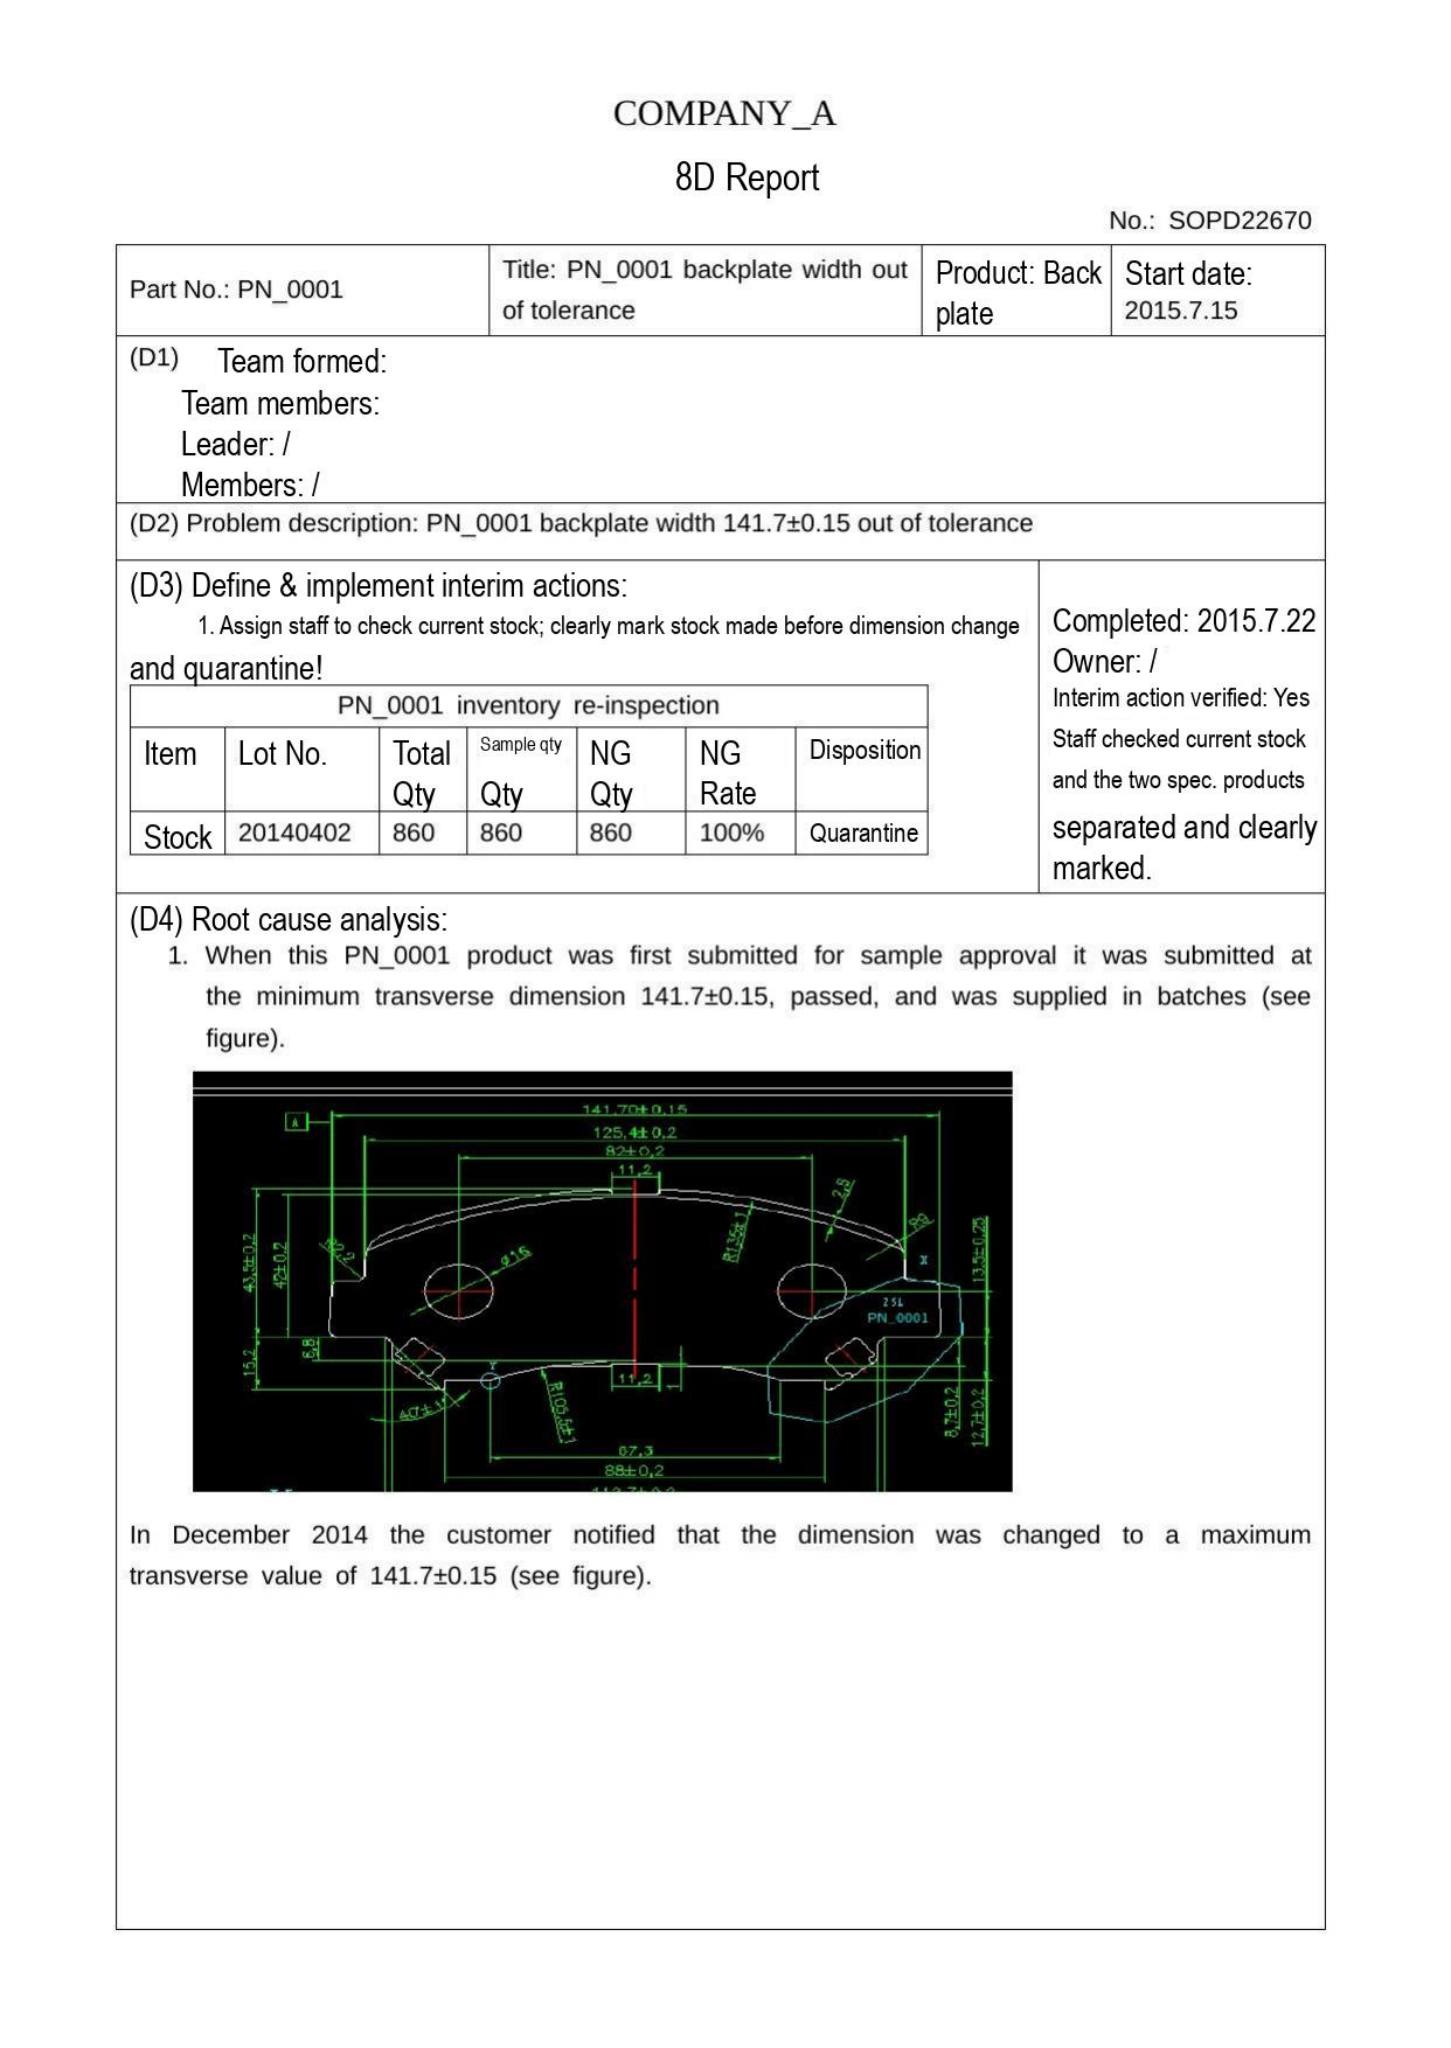COMPANY_A

8D Report

No.: SOPD22670

| Part No.: PN_0001 | Title: PN_0001 backplate width out of tolerance | Product: Back plate | Start date: 2015.7.15 |
|---|---|---|---|

(D1) Team formed:
Team members:
Leader: /
Members: /

(D2) Problem description: PN_0001 backplate width 141.7±0.15 out of tolerance

(D3) Define & implement interim actions:
1. Assign staff to check current stock; clearly mark stock made before dimension change and quarantine!

PN_0001 inventory re-inspection

| Item | Lot No. | Total Qty | Sample qty Qty | NG Qty | NG Rate | Disposition |
|---|---|---|---|---|---|---|
| Stock | 20140402 | 860 | 860 | 860 | 100% | Quarantine |

Completed: 2015.7.22
Owner: /
Interim action verified: Yes
Staff checked current stock and the two spec. products separated and clearly marked.

(D4) Root cause analysis:
1. When this PN_0001 product was first submitted for sample approval it was submitted at the minimum transverse dimension 141.7±0.15, passed, and was supplied in batches (see figure).

A
141.70±0.15
125.4±0.2
82±0.2
11.2
2.5
ø15
R135±1
43.5±0.2
42±0.2
13.5±0.25
PN_0001
6.8
15.2
11.2
R100±1
40±1
8.7±0.2
12.7±0.2
67.3
88±0.2

In December 2014 the customer notified that the dimension was changed to a maximum transverse value of 141.7±0.15 (see figure).
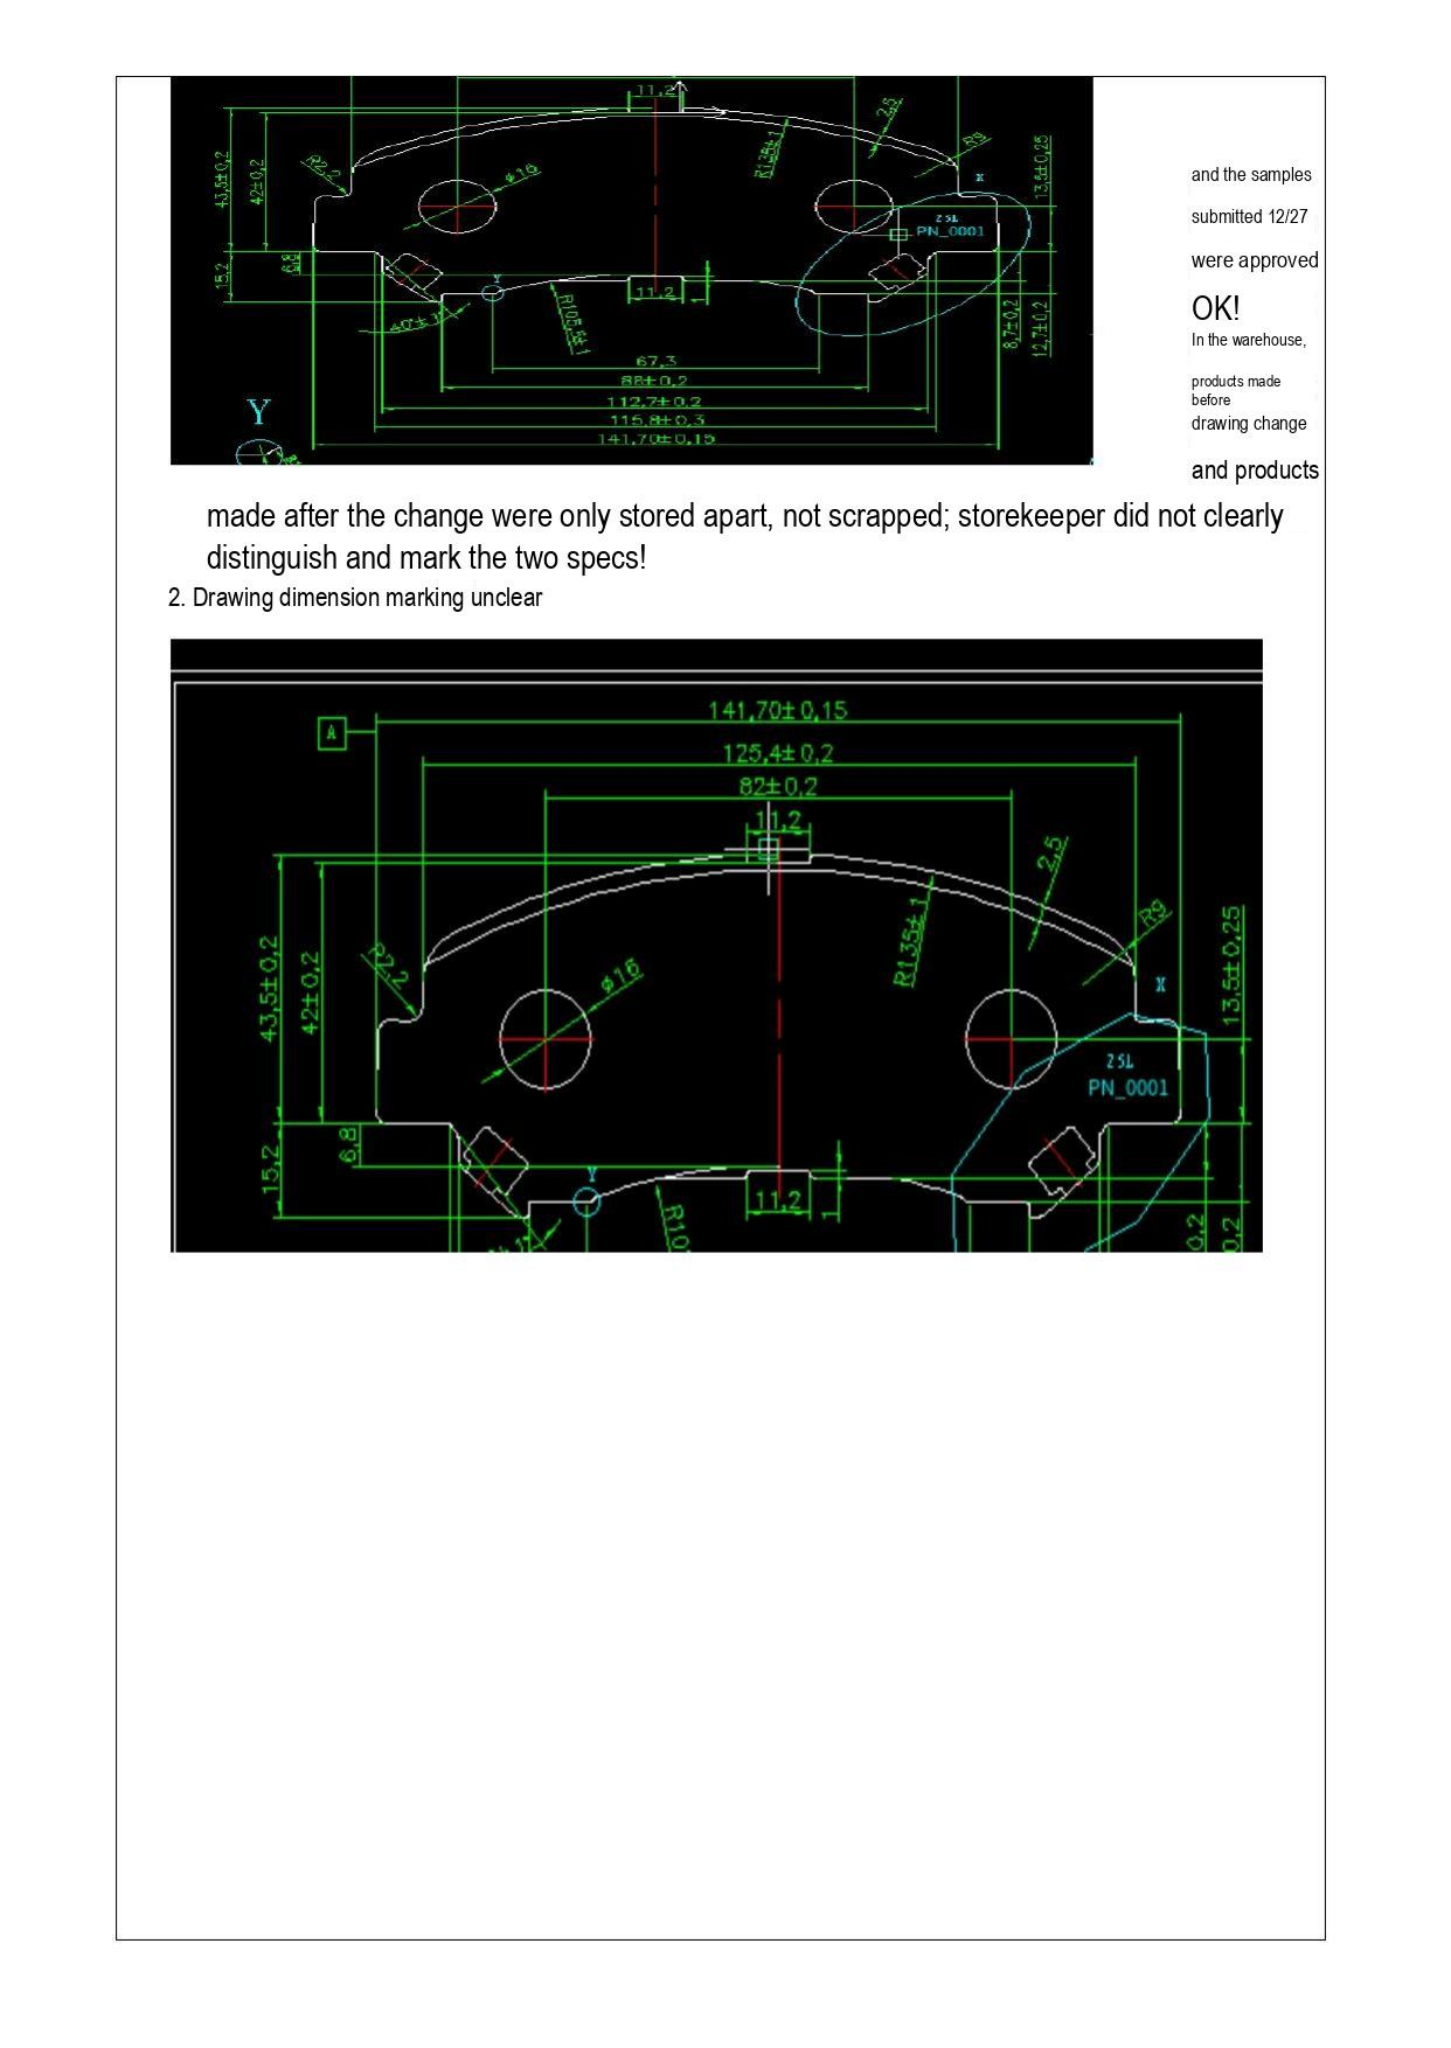11,2
2,5
R135±1
R9
R2,0
ϕ16
43,5±0,2
42±0,2
13,5±0,25
X
Z5L
PN_0001
15,2
6,8
Y
11,2
R105,5±1
40±1
8,7±0,2
12,7±0,2
67,3
88±0,2
112,7±0,2
115,8±0,3
141,70±0,15
Y

and the samples
submitted 12/27
were approved
OK!
In the warehouse,
products made before
drawing change
and products
made after the change were only stored apart, not scrapped; storekeeper did not clearly distinguish and mark the two specs!

2. Drawing dimension marking unclear

A
141,70±0,15
125,4±0,2
82±0,2
11,2
2,5
R135±1
R9
R2,2
ϕ16
43,5±0,2
42±0,2
13,5±0,25
X
Z5L
PN_0001
15,2
6,8
Y
11,2
1
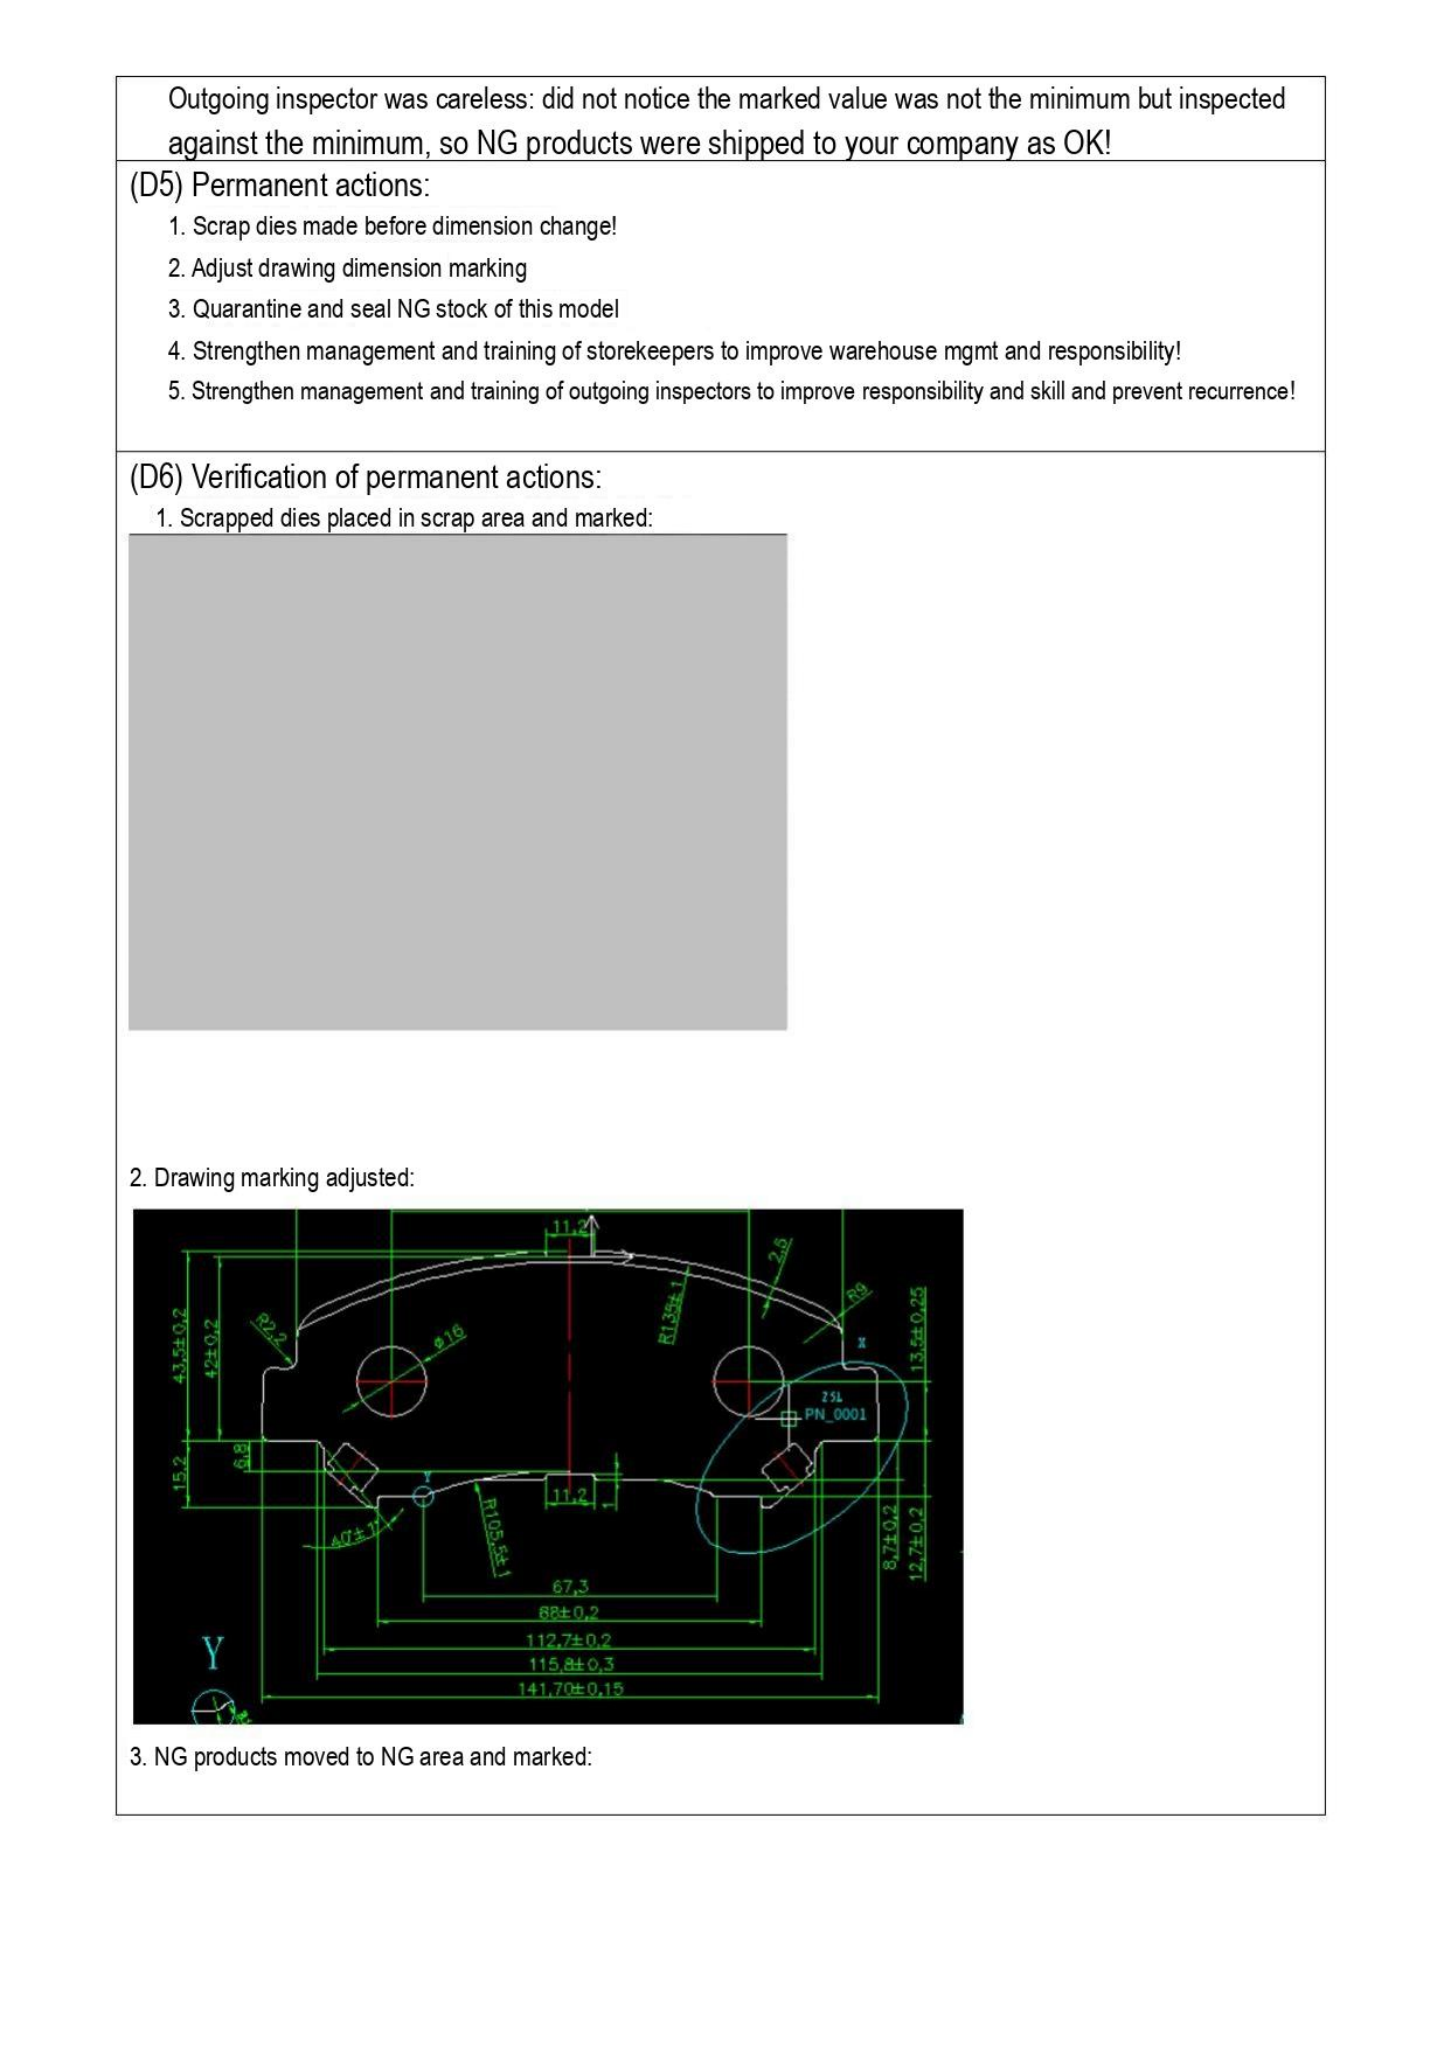Outgoing inspector was careless: did not notice the marked value was not the minimum but inspected against the minimum, so NG products were shipped to your company as OK!

(D5) Permanent actions:

1. Scrap dies made before dimension change!
2. Adjust drawing dimension marking
3. Quarantine and seal NG stock of this model
4. Strengthen management and training of storekeepers to improve warehouse mgmt and responsibility!
5. Strengthen management and training of outgoing inspectors to improve responsibility and skill and prevent recurrence!

(D6) Verification of permanent actions:

1. Scrapped dies placed in scrap area and marked:

2. Drawing marking adjusted:

11,2
2,6
R139±1
R9
43,5±0,2
42±0,2
R2,2
ø16
13,5±0,25
X
25L
PN_0001
15,2
6,8
Y
11,2
R105,5±1
40°±1°
8,7±0,2
12,7±0,2
67,3
88±0,2
112,7±0,2
115,8±0,3
141,70±0,15
Y

3. NG products moved to NG area and marked:
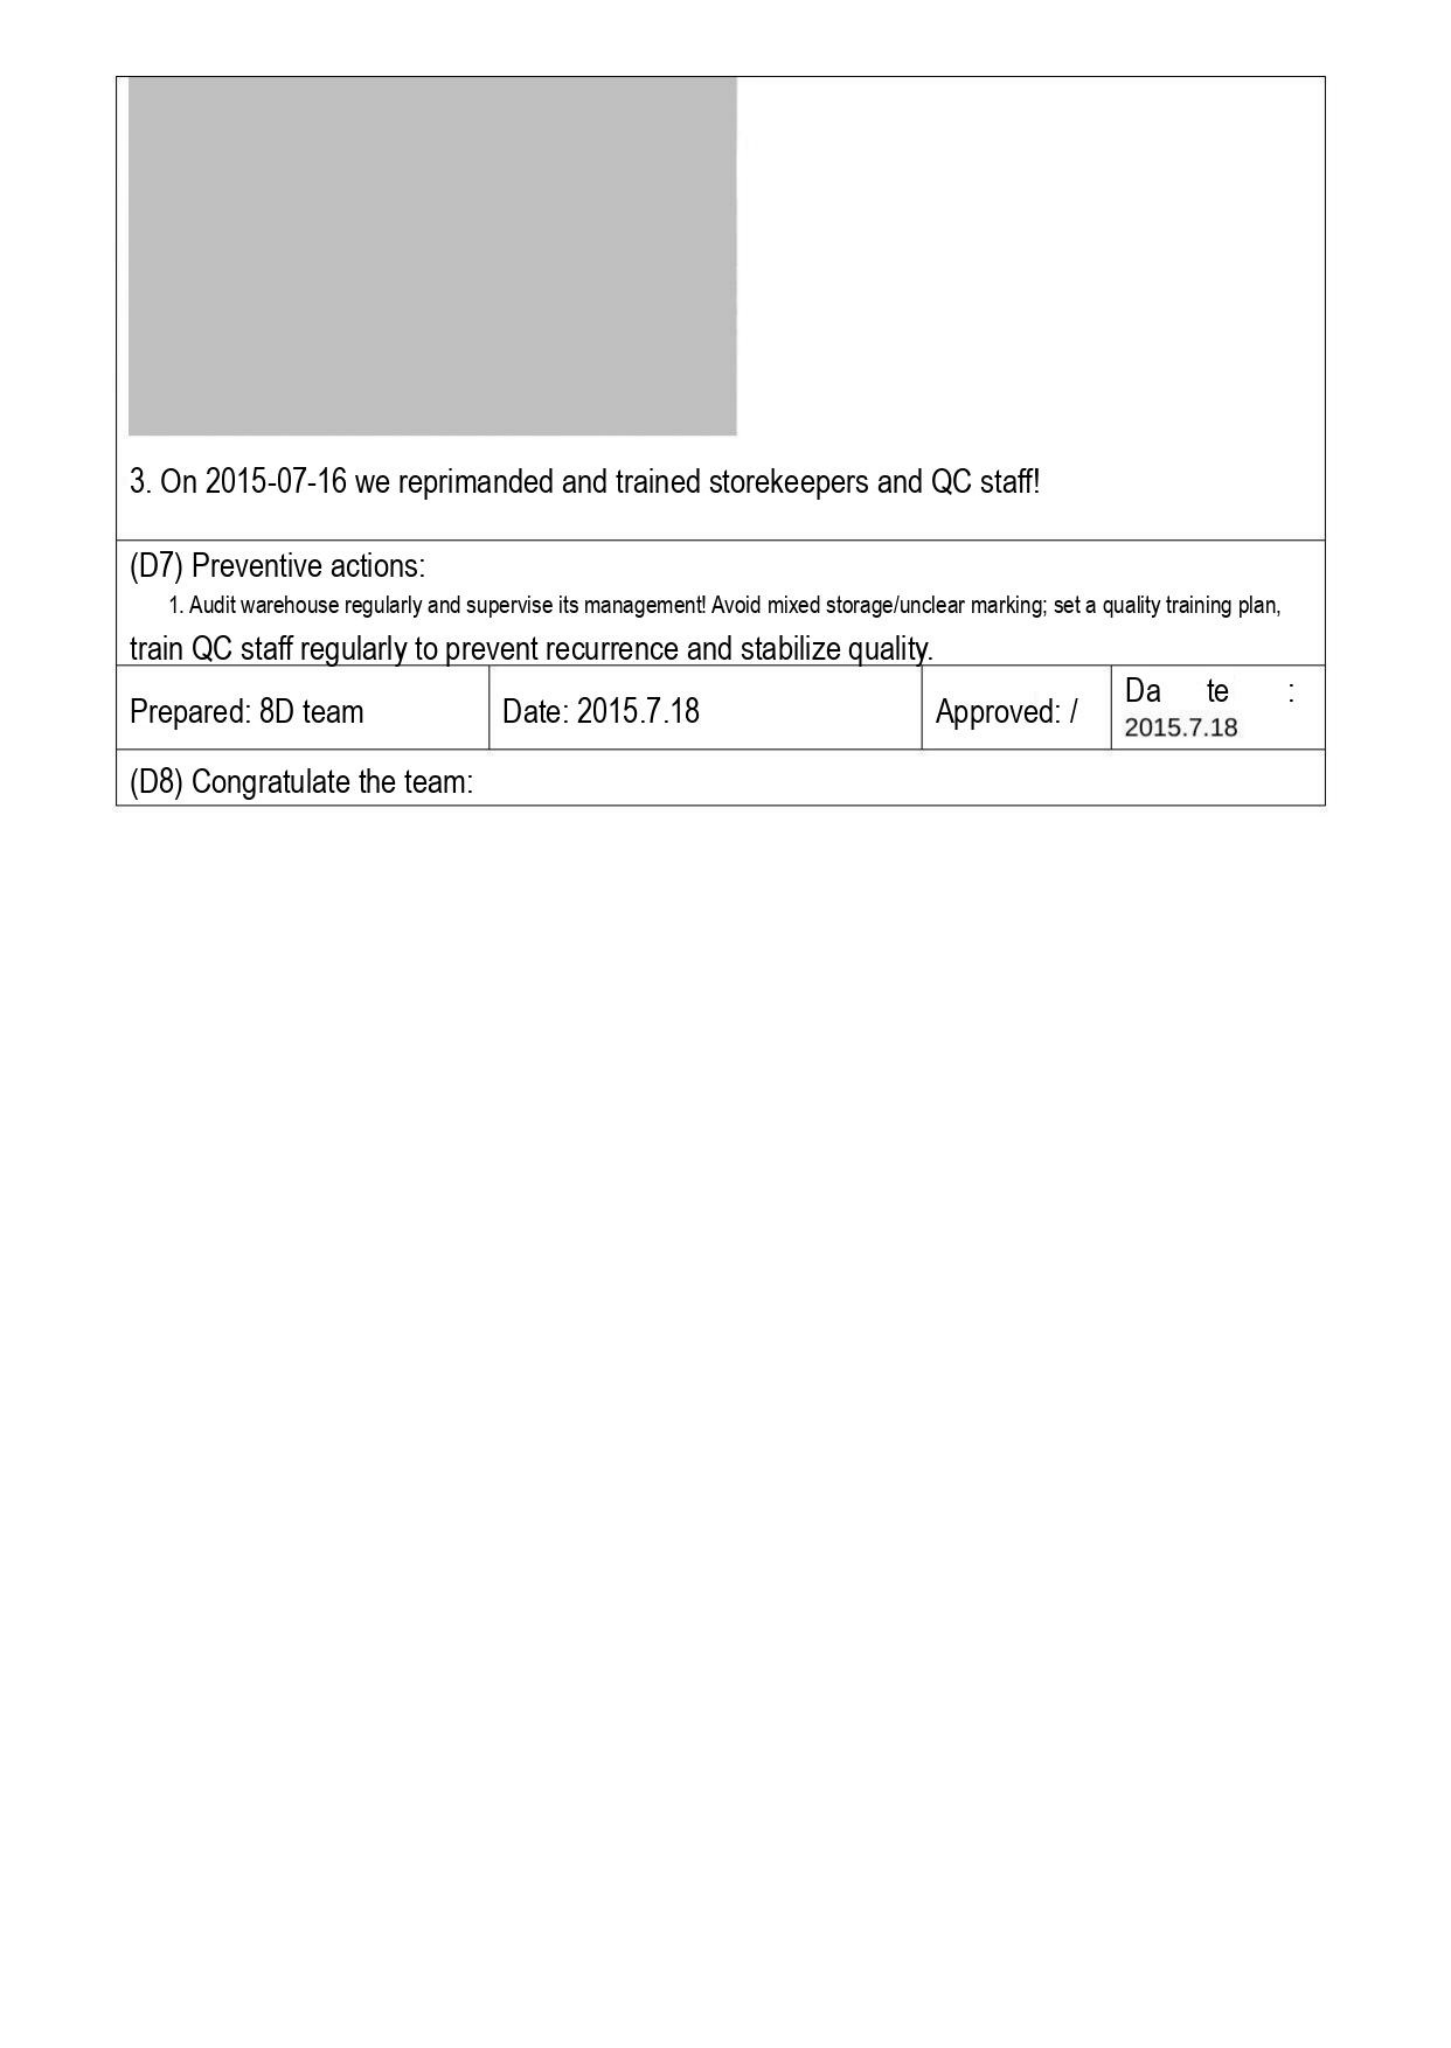3. On 2015-07-16 we reprimanded and trained storekeepers and QC staff!

(D7) Preventive actions:

1. Audit warehouse regularly and supervise its management! Avoid mixed storage/unclear marking; set a quality training plan, train QC staff regularly to prevent recurrence and stabilize quality.

| Prepared: 8D team | Date: 2015.7.18 | Approved: / | Date: 2015.7.18 |
|---|---|---|---|

(D8) Congratulate the team: